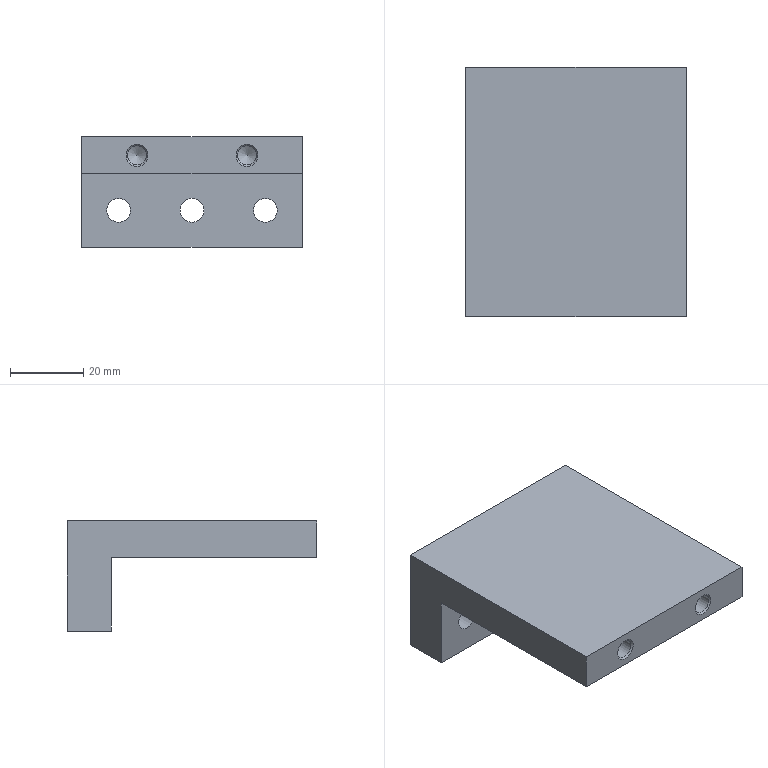Part | NX | features SIMPLE HOLE 5, DATUM_CSYS 4, SKETCH 3, HOLE PACKAGE 2, SYMBOLIC_THREAD 2, EXTRUDE 1 | 1 solid | 17 faces | box 60 x 68 x 30 mm | volume 53216 mm3 | plane 8 | cylinder 5 | cone 4 | commonest cylinder face diameters 6.5 x3 5.2 x2
STEP:
#1=CARTESIAN_POINT('',(15.,-68.,28.));
#2=VERTEX_POINT('',#1);
#3=CARTESIAN_POINT('',(15.,-68.,25.));
#4=DIRECTION('',(0.,1.,0.));
#5=DIRECTION('',(0.,0.,1.));
#6=AXIS2_PLACEMENT_3D('',#3,#4,#5);
#7=CIRCLE('',#6,3.);
#8=EDGE_CURVE('',#2,#2,#7,.T.);
#9=ORIENTED_EDGE('',*,*,#8,.T.);
#10=EDGE_LOOP('',(#9));
#11=FACE_BOUND('',#10,.T.);
#12=CARTESIAN_POINT('',(-15.,-68.,28.));
#13=VERTEX_POINT('',#12);
#14=CARTESIAN_POINT('',(-15.,-68.,25.));
#15=DIRECTION('',(0.,1.,0.));
#16=DIRECTION('',(0.,0.,1.));
#17=AXIS2_PLACEMENT_3D('',#14,#15,#16);
#18=CIRCLE('',#17,3.);
#19=EDGE_CURVE('',#13,#13,#18,.T.);
#20=ORIENTED_EDGE('',*,*,#19,.T.);
#21=EDGE_LOOP('',(#20));
#22=FACE_BOUND('',#21,.T.);
#23=CARTESIAN_POINT('',(-30.,-68.,30.));
#24=VERTEX_POINT('',#23);
#25=CARTESIAN_POINT('',(-30.,-68.,20.));
#26=VERTEX_POINT('',#25);
#27=CARTESIAN_POINT('',(-30.,-68.,30.));
#28=DIRECTION('',(0.,0.,-1.));
#29=VECTOR('',#28,1000.);
#30=LINE('',#27,#29);
#31=EDGE_CURVE('',#24,#26,#30,.T.);
#32=ORIENTED_EDGE('',*,*,#31,.T.);
#33=CARTESIAN_POINT('',(30.,-68.,20.));
#34=VERTEX_POINT('',#33);
#35=CARTESIAN_POINT('',(30.,-68.,20.));
#36=DIRECTION('',(-1.,0.,0.));
#37=VECTOR('',#36,1000.);
#38=LINE('',#35,#37);
#39=EDGE_CURVE('',#34,#26,#38,.T.);
#40=ORIENTED_EDGE('',*,*,#39,.F.);
#41=CARTESIAN_POINT('',(30.,-68.,30.));
#42=VERTEX_POINT('',#41);
#43=CARTESIAN_POINT('',(30.,-68.,30.));
#44=DIRECTION('',(0.,0.,-1.));
#45=VECTOR('',#44,1000.);
#46=LINE('',#43,#45);
#47=EDGE_CURVE('',#42,#34,#46,.T.);
#48=ORIENTED_EDGE('',*,*,#47,.F.);
#49=CARTESIAN_POINT('',(30.,-68.,30.));
#50=DIRECTION('',(-1.,0.,0.));
#51=VECTOR('',#50,1000.);
#52=LINE('',#49,#51);
#53=EDGE_CURVE('',#42,#24,#52,.T.);
#54=ORIENTED_EDGE('',*,*,#53,.T.);
#55=EDGE_LOOP('',(#32,#40,#48,#54));
#56=FACE_BOUND('',#55,.T.);
#57=CARTESIAN_POINT('',(30.,-68.,30.));
#58=DIRECTION('',(0.,1.,0.));
#59=DIRECTION('',(0.,0.,1.));
#60=AXIS2_PLACEMENT_3D('',#57,#58,#59);
#61=PLANE('',#60);
#62=ADVANCED_FACE('',(#11,#22,#56),#61,.F.);
#63=CARTESIAN_POINT('',(-30.,-12.,20.));
#64=VERTEX_POINT('',#63);
#65=CARTESIAN_POINT('',(-30.,-68.,20.));
#66=DIRECTION('',(0.,1.,0.));
#67=VECTOR('',#66,1000.);
#68=LINE('',#65,#67);
#69=EDGE_CURVE('',#26,#64,#68,.T.);
#70=ORIENTED_EDGE('',*,*,#69,.T.);
#71=CARTESIAN_POINT('',(30.,-12.,20.));
#72=VERTEX_POINT('',#71);
#73=CARTESIAN_POINT('',(30.,-12.,20.));
#74=DIRECTION('',(-1.,0.,0.));
#75=VECTOR('',#74,1000.);
#76=LINE('',#73,#75);
#77=EDGE_CURVE('',#72,#64,#76,.T.);
#78=ORIENTED_EDGE('',*,*,#77,.F.);
#79=CARTESIAN_POINT('',(30.,-68.,20.));
#80=DIRECTION('',(0.,1.,0.));
#81=VECTOR('',#80,1000.);
#82=LINE('',#79,#81);
#83=EDGE_CURVE('',#34,#72,#82,.T.);
#84=ORIENTED_EDGE('',*,*,#83,.F.);
#85=ORIENTED_EDGE('',*,*,#39,.T.);
#86=EDGE_LOOP('',(#70,#78,#84,#85));
#87=FACE_BOUND('',#86,.T.);
#88=CARTESIAN_POINT('',(30.,-68.,20.));
#89=DIRECTION('',(0.,0.,1.));
#90=DIRECTION('',(1.,0.,0.));
#91=AXIS2_PLACEMENT_3D('',#88,#89,#90);
#92=PLANE('',#91);
#93=ADVANCED_FACE('',(#87),#92,.F.);
#94=CARTESIAN_POINT('',(-20.,-12.,13.25));
#95=VERTEX_POINT('',#94);
#96=CARTESIAN_POINT('',(-20.,-12.,10.));
#97=DIRECTION('',(0.,1.,0.));
#98=DIRECTION('',(0.,0.,1.));
#99=AXIS2_PLACEMENT_3D('',#96,#97,#98);
#100=CIRCLE('',#99,3.25);
#101=EDGE_CURVE('',#95,#95,#100,.T.);
#102=ORIENTED_EDGE('',*,*,#101,.T.);
#103=EDGE_LOOP('',(#102));
#104=FACE_BOUND('',#103,.T.);
#105=CARTESIAN_POINT('',(0.,-12.,13.25));
#106=VERTEX_POINT('',#105);
#107=CARTESIAN_POINT('',(0.,-12.,10.));
#108=DIRECTION('',(0.,1.,0.));
#109=DIRECTION('',(0.,0.,1.));
#110=AXIS2_PLACEMENT_3D('',#107,#108,#109);
#111=CIRCLE('',#110,3.25);
#112=EDGE_CURVE('',#106,#106,#111,.T.);
#113=ORIENTED_EDGE('',*,*,#112,.T.);
#114=EDGE_LOOP('',(#113));
#115=FACE_BOUND('',#114,.T.);
#116=CARTESIAN_POINT('',(20.,-12.,13.25));
#117=VERTEX_POINT('',#116);
#118=CARTESIAN_POINT('',(20.,-12.,10.));
#119=DIRECTION('',(0.,1.,0.));
#120=DIRECTION('',(0.,0.,1.));
#121=AXIS2_PLACEMENT_3D('',#118,#119,#120);
#122=CIRCLE('',#121,3.25);
#123=EDGE_CURVE('',#117,#117,#122,.T.);
#124=ORIENTED_EDGE('',*,*,#123,.T.);
#125=EDGE_LOOP('',(#124));
#126=FACE_BOUND('',#125,.T.);
#127=CARTESIAN_POINT('',(-30.,-12.,0.));
#128=VERTEX_POINT('',#127);
#129=CARTESIAN_POINT('',(-30.,-12.,20.));
#130=DIRECTION('',(0.,0.,-1.));
#131=VECTOR('',#130,1000.);
#132=LINE('',#129,#131);
#133=EDGE_CURVE('',#64,#128,#132,.T.);
#134=ORIENTED_EDGE('',*,*,#133,.T.);
#135=CARTESIAN_POINT('',(30.,-12.,0.));
#136=VERTEX_POINT('',#135);
#137=CARTESIAN_POINT('',(30.,-12.,0.));
#138=DIRECTION('',(-1.,0.,0.));
#139=VECTOR('',#138,1000.);
#140=LINE('',#137,#139);
#141=EDGE_CURVE('',#136,#128,#140,.T.);
#142=ORIENTED_EDGE('',*,*,#141,.F.);
#143=CARTESIAN_POINT('',(30.,-12.,20.));
#144=DIRECTION('',(0.,0.,-1.));
#145=VECTOR('',#144,1000.);
#146=LINE('',#143,#145);
#147=EDGE_CURVE('',#72,#136,#146,.T.);
#148=ORIENTED_EDGE('',*,*,#147,.F.);
#149=ORIENTED_EDGE('',*,*,#77,.T.);
#150=EDGE_LOOP('',(#134,#142,#148,#149));
#151=FACE_BOUND('',#150,.T.);
#152=CARTESIAN_POINT('',(30.,-12.,20.));
#153=DIRECTION('',(0.,1.,0.));
#154=DIRECTION('',(0.,0.,1.));
#155=AXIS2_PLACEMENT_3D('',#152,#153,#154);
#156=PLANE('',#155);
#157=ADVANCED_FACE('',(#104,#115,#126,#151),#156,.F.);
#158=CARTESIAN_POINT('',(-30.,0.,0.));
#159=VERTEX_POINT('',#158);
#160=CARTESIAN_POINT('',(-30.,-12.,0.));
#161=DIRECTION('',(0.,1.,0.));
#162=VECTOR('',#161,1000.);
#163=LINE('',#160,#162);
#164=EDGE_CURVE('',#128,#159,#163,.T.);
#165=ORIENTED_EDGE('',*,*,#164,.T.);
#166=CARTESIAN_POINT('',(30.,0.,0.));
#167=VERTEX_POINT('',#166);
#168=CARTESIAN_POINT('',(30.,0.,0.));
#169=DIRECTION('',(-1.,0.,0.));
#170=VECTOR('',#169,1000.);
#171=LINE('',#168,#170);
#172=EDGE_CURVE('',#167,#159,#171,.T.);
#173=ORIENTED_EDGE('',*,*,#172,.F.);
#174=CARTESIAN_POINT('',(30.,-12.,0.));
#175=DIRECTION('',(0.,1.,0.));
#176=VECTOR('',#175,1000.);
#177=LINE('',#174,#176);
#178=EDGE_CURVE('',#136,#167,#177,.T.);
#179=ORIENTED_EDGE('',*,*,#178,.F.);
#180=ORIENTED_EDGE('',*,*,#141,.T.);
#181=EDGE_LOOP('',(#165,#173,#179,#180));
#182=FACE_BOUND('',#181,.T.);
#183=CARTESIAN_POINT('',(30.,-12.,0.));
#184=DIRECTION('',(0.,0.,1.));
#185=DIRECTION('',(1.,0.,0.));
#186=AXIS2_PLACEMENT_3D('',#183,#184,#185);
#187=PLANE('',#186);
#188=ADVANCED_FACE('',(#182),#187,.F.);
#189=CARTESIAN_POINT('',(-20.,0.,6.75));
#190=VERTEX_POINT('',#189);
#191=CARTESIAN_POINT('',(-20.,0.,10.));
#192=DIRECTION('',(0.,-1.,0.));
#193=DIRECTION('',(0.,0.,-1.));
#194=AXIS2_PLACEMENT_3D('',#191,#192,#193);
#195=CIRCLE('',#194,3.25);
#196=EDGE_CURVE('',#190,#190,#195,.T.);
#197=ORIENTED_EDGE('',*,*,#196,.T.);
#198=EDGE_LOOP('',(#197));
#199=FACE_BOUND('',#198,.T.);
#200=CARTESIAN_POINT('',(0.,0.,6.75));
#201=VERTEX_POINT('',#200);
#202=CARTESIAN_POINT('',(0.,0.,10.));
#203=DIRECTION('',(0.,-1.,0.));
#204=DIRECTION('',(0.,0.,-1.));
#205=AXIS2_PLACEMENT_3D('',#202,#203,#204);
#206=CIRCLE('',#205,3.25);
#207=EDGE_CURVE('',#201,#201,#206,.T.);
#208=ORIENTED_EDGE('',*,*,#207,.T.);
#209=EDGE_LOOP('',(#208));
#210=FACE_BOUND('',#209,.T.);
#211=CARTESIAN_POINT('',(20.,0.,6.75));
#212=VERTEX_POINT('',#211);
#213=CARTESIAN_POINT('',(20.,0.,10.));
#214=DIRECTION('',(0.,-1.,0.));
#215=DIRECTION('',(0.,0.,-1.));
#216=AXIS2_PLACEMENT_3D('',#213,#214,#215);
#217=CIRCLE('',#216,3.25);
#218=EDGE_CURVE('',#212,#212,#217,.T.);
#219=ORIENTED_EDGE('',*,*,#218,.T.);
#220=EDGE_LOOP('',(#219));
#221=FACE_BOUND('',#220,.T.);
#222=CARTESIAN_POINT('',(-30.,0.,30.));
#223=VERTEX_POINT('',#222);
#224=CARTESIAN_POINT('',(-30.,0.,0.));
#225=DIRECTION('',(0.,0.,1.));
#226=VECTOR('',#225,1000.);
#227=LINE('',#224,#226);
#228=EDGE_CURVE('',#159,#223,#227,.T.);
#229=ORIENTED_EDGE('',*,*,#228,.T.);
#230=CARTESIAN_POINT('',(30.,0.,30.));
#231=VERTEX_POINT('',#230);
#232=CARTESIAN_POINT('',(30.,0.,30.));
#233=DIRECTION('',(-1.,0.,0.));
#234=VECTOR('',#233,1000.);
#235=LINE('',#232,#234);
#236=EDGE_CURVE('',#231,#223,#235,.T.);
#237=ORIENTED_EDGE('',*,*,#236,.F.);
#238=CARTESIAN_POINT('',(30.,0.,0.));
#239=DIRECTION('',(0.,0.,1.));
#240=VECTOR('',#239,1000.);
#241=LINE('',#238,#240);
#242=EDGE_CURVE('',#167,#231,#241,.T.);
#243=ORIENTED_EDGE('',*,*,#242,.F.);
#244=ORIENTED_EDGE('',*,*,#172,.T.);
#245=EDGE_LOOP('',(#229,#237,#243,#244));
#246=FACE_BOUND('',#245,.T.);
#247=CARTESIAN_POINT('',(30.,0.,0.));
#248=DIRECTION('',(0.,-1.,0.));
#249=DIRECTION('',(0.,0.,-1.));
#250=AXIS2_PLACEMENT_3D('',#247,#248,#249);
#251=PLANE('',#250);
#252=ADVANCED_FACE('',(#199,#210,#221,#246),#251,.F.);
#253=CARTESIAN_POINT('',(-30.,0.,30.));
#254=DIRECTION('',(0.,-1.,0.));
#255=VECTOR('',#254,1000.);
#256=LINE('',#253,#255);
#257=EDGE_CURVE('',#223,#24,#256,.T.);
#258=ORIENTED_EDGE('',*,*,#257,.T.);
#259=ORIENTED_EDGE('',*,*,#53,.F.);
#260=CARTESIAN_POINT('',(30.,0.,30.));
#261=DIRECTION('',(0.,-1.,0.));
#262=VECTOR('',#261,1000.);
#263=LINE('',#260,#262);
#264=EDGE_CURVE('',#231,#42,#263,.T.);
#265=ORIENTED_EDGE('',*,*,#264,.F.);
#266=ORIENTED_EDGE('',*,*,#236,.T.);
#267=EDGE_LOOP('',(#258,#259,#265,#266));
#268=FACE_BOUND('',#267,.T.);
#269=CARTESIAN_POINT('',(30.,0.,30.));
#270=DIRECTION('',(0.,0.,-1.));
#271=DIRECTION('',(0.,1.,0.));
#272=AXIS2_PLACEMENT_3D('',#269,#270,#271);
#273=PLANE('',#272);
#274=ADVANCED_FACE('',(#268),#273,.F.);
#275=ORIENTED_EDGE('',*,*,#47,.T.);
#276=ORIENTED_EDGE('',*,*,#83,.T.);
#277=ORIENTED_EDGE('',*,*,#147,.T.);
#278=ORIENTED_EDGE('',*,*,#178,.T.);
#279=ORIENTED_EDGE('',*,*,#242,.T.);
#280=ORIENTED_EDGE('',*,*,#264,.T.);
#281=EDGE_LOOP('',(#275,#276,#277,#278,#279,#280));
#282=FACE_BOUND('',#281,.T.);
#283=CARTESIAN_POINT('',(30.,0.,0.));
#284=DIRECTION('',(1.,0.,0.));
#285=DIRECTION('',(0.,0.,-1.));
#286=AXIS2_PLACEMENT_3D('',#283,#284,#285);
#287=PLANE('',#286);
#288=ADVANCED_FACE('',(#282),#287,.T.);
#289=ORIENTED_EDGE('',*,*,#31,.F.);
#290=ORIENTED_EDGE('',*,*,#257,.F.);
#291=ORIENTED_EDGE('',*,*,#228,.F.);
#292=ORIENTED_EDGE('',*,*,#164,.F.);
#293=ORIENTED_EDGE('',*,*,#133,.F.);
#294=ORIENTED_EDGE('',*,*,#69,.F.);
#295=EDGE_LOOP('',(#289,#290,#291,#292,#293,#294));
#296=FACE_BOUND('',#295,.T.);
#297=CARTESIAN_POINT('',(-30.,0.,0.));
#298=DIRECTION('',(1.,0.,0.));
#299=DIRECTION('',(0.,0.,-1.));
#300=AXIS2_PLACEMENT_3D('',#297,#298,#299);
#301=PLANE('',#300);
#302=ADVANCED_FACE('',(#296),#301,.F.);
#303=CARTESIAN_POINT('',(-15.,-50.,27.6));
#304=VERTEX_POINT('',#303);
#305=CARTESIAN_POINT('',(-15.,-50.,25.));
#306=DIRECTION('',(0.,1.,0.));
#307=DIRECTION('',(0.,0.,1.));
#308=AXIS2_PLACEMENT_3D('',#305,#306,#307);
#309=CIRCLE('',#308,2.6);
#310=EDGE_CURVE('',#304,#304,#309,.F.);
#311=ORIENTED_EDGE('',*,*,#310,.T.);
#312=EDGE_LOOP('',(#311));
#313=FACE_BOUND('',#312,.T.);
#314=CARTESIAN_POINT('',(-15.,-48.438,25.));
#315=VERTEX_POINT('',#314);
#316=VERTEX_LOOP('',#315);
#317=FACE_BOUND('',#316,.T.);
#318=CARTESIAN_POINT('',(-15.,-50.,25.));
#319=DIRECTION('',(0.,-1.,0.));
#320=DIRECTION('',(0.,0.,-1.));
#321=AXIS2_PLACEMENT_3D('',#318,#319,#320);
#322=CONICAL_SURFACE('',#321,2.6,1.03);
#323=ADVANCED_FACE('',(#313,#317),#322,.F.);
#324=CARTESIAN_POINT('',(-15.,-67.6,27.6));
#325=VERTEX_POINT('',#324);
#326=CARTESIAN_POINT('',(-15.,-67.6,25.));
#327=DIRECTION('',(0.,1.,0.));
#328=DIRECTION('',(0.,0.,1.));
#329=AXIS2_PLACEMENT_3D('',#326,#327,#328);
#330=CIRCLE('',#329,2.6);
#331=EDGE_CURVE('',#325,#325,#330,.F.);
#332=ORIENTED_EDGE('',*,*,#331,.T.);
#333=EDGE_LOOP('',(#332));
#334=FACE_BOUND('',#333,.T.);
#335=ORIENTED_EDGE('',*,*,#310,.F.);
#336=EDGE_LOOP('',(#335));
#337=FACE_BOUND('',#336,.T.);
#338=CARTESIAN_POINT('',(-15.,-68.,25.));
#339=DIRECTION('',(0.,1.,0.));
#340=DIRECTION('',(0.,0.,1.));
#341=AXIS2_PLACEMENT_3D('',#338,#339,#340);
#342=CYLINDRICAL_SURFACE('',#341,2.6);
#343=ADVANCED_FACE('',(#334,#337),#342,.F.);
#344=ORIENTED_EDGE('',*,*,#331,.F.);
#345=EDGE_LOOP('',(#344));
#346=FACE_BOUND('',#345,.T.);
#347=ORIENTED_EDGE('',*,*,#19,.F.);
#348=EDGE_LOOP('',(#347));
#349=FACE_BOUND('',#348,.T.);
#350=CARTESIAN_POINT('',(-15.,-68.,25.));
#351=DIRECTION('',(0.,-1.,0.));
#352=DIRECTION('',(0.,0.,-1.));
#353=AXIS2_PLACEMENT_3D('',#350,#351,#352);
#354=CONICAL_SURFACE('',#353,3.,0.7854);
#355=ADVANCED_FACE('',(#346,#349),#354,.F.);
#356=CARTESIAN_POINT('',(15.,-50.,27.6));
#357=VERTEX_POINT('',#356);
#358=CARTESIAN_POINT('',(15.,-50.,25.));
#359=DIRECTION('',(0.,1.,0.));
#360=DIRECTION('',(0.,0.,1.));
#361=AXIS2_PLACEMENT_3D('',#358,#359,#360);
#362=CIRCLE('',#361,2.6);
#363=EDGE_CURVE('',#357,#357,#362,.F.);
#364=ORIENTED_EDGE('',*,*,#363,.T.);
#365=EDGE_LOOP('',(#364));
#366=FACE_BOUND('',#365,.T.);
#367=CARTESIAN_POINT('',(15.,-48.438,25.));
#368=VERTEX_POINT('',#367);
#369=VERTEX_LOOP('',#368);
#370=FACE_BOUND('',#369,.T.);
#371=CARTESIAN_POINT('',(15.,-50.,25.));
#372=DIRECTION('',(0.,-1.,0.));
#373=DIRECTION('',(0.,0.,-1.));
#374=AXIS2_PLACEMENT_3D('',#371,#372,#373);
#375=CONICAL_SURFACE('',#374,2.6,1.03);
#376=ADVANCED_FACE('',(#366,#370),#375,.F.);
#377=CARTESIAN_POINT('',(15.,-67.6,27.6));
#378=VERTEX_POINT('',#377);
#379=CARTESIAN_POINT('',(15.,-67.6,25.));
#380=DIRECTION('',(0.,1.,0.));
#381=DIRECTION('',(0.,0.,1.));
#382=AXIS2_PLACEMENT_3D('',#379,#380,#381);
#383=CIRCLE('',#382,2.6);
#384=EDGE_CURVE('',#378,#378,#383,.F.);
#385=ORIENTED_EDGE('',*,*,#384,.T.);
#386=EDGE_LOOP('',(#385));
#387=FACE_BOUND('',#386,.T.);
#388=ORIENTED_EDGE('',*,*,#363,.F.);
#389=EDGE_LOOP('',(#388));
#390=FACE_BOUND('',#389,.T.);
#391=CARTESIAN_POINT('',(15.,-68.,25.));
#392=DIRECTION('',(0.,1.,0.));
#393=DIRECTION('',(0.,0.,1.));
#394=AXIS2_PLACEMENT_3D('',#391,#392,#393);
#395=CYLINDRICAL_SURFACE('',#394,2.6);
#396=ADVANCED_FACE('',(#387,#390),#395,.F.);
#397=ORIENTED_EDGE('',*,*,#384,.F.);
#398=EDGE_LOOP('',(#397));
#399=FACE_BOUND('',#398,.T.);
#400=ORIENTED_EDGE('',*,*,#8,.F.);
#401=EDGE_LOOP('',(#400));
#402=FACE_BOUND('',#401,.T.);
#403=CARTESIAN_POINT('',(15.,-68.,25.));
#404=DIRECTION('',(0.,-1.,0.));
#405=DIRECTION('',(0.,0.,-1.));
#406=AXIS2_PLACEMENT_3D('',#403,#404,#405);
#407=CONICAL_SURFACE('',#406,3.,0.7854);
#408=ADVANCED_FACE('',(#399,#402),#407,.F.);
#409=ORIENTED_EDGE('',*,*,#123,.F.);
#410=EDGE_LOOP('',(#409));
#411=FACE_BOUND('',#410,.T.);
#412=ORIENTED_EDGE('',*,*,#218,.F.);
#413=EDGE_LOOP('',(#412));
#414=FACE_BOUND('',#413,.T.);
#415=CARTESIAN_POINT('',(20.,-12.,10.));
#416=DIRECTION('',(0.,1.,0.));
#417=DIRECTION('',(0.,0.,1.));
#418=AXIS2_PLACEMENT_3D('',#415,#416,#417);
#419=CYLINDRICAL_SURFACE('',#418,3.25);
#420=ADVANCED_FACE('',(#411,#414),#419,.F.);
#421=ORIENTED_EDGE('',*,*,#112,.F.);
#422=EDGE_LOOP('',(#421));
#423=FACE_BOUND('',#422,.T.);
#424=ORIENTED_EDGE('',*,*,#207,.F.);
#425=EDGE_LOOP('',(#424));
#426=FACE_BOUND('',#425,.T.);
#427=CARTESIAN_POINT('',(0.,-12.,10.));
#428=DIRECTION('',(0.,1.,0.));
#429=DIRECTION('',(0.,0.,1.));
#430=AXIS2_PLACEMENT_3D('',#427,#428,#429);
#431=CYLINDRICAL_SURFACE('',#430,3.25);
#432=ADVANCED_FACE('',(#423,#426),#431,.F.);
#433=ORIENTED_EDGE('',*,*,#101,.F.);
#434=EDGE_LOOP('',(#433));
#435=FACE_BOUND('',#434,.T.);
#436=ORIENTED_EDGE('',*,*,#196,.F.);
#437=EDGE_LOOP('',(#436));
#438=FACE_BOUND('',#437,.T.);
#439=CARTESIAN_POINT('',(-20.,-12.,10.));
#440=DIRECTION('',(0.,1.,0.));
#441=DIRECTION('',(0.,0.,1.));
#442=AXIS2_PLACEMENT_3D('',#439,#440,#441);
#443=CYLINDRICAL_SURFACE('',#442,3.25);
#444=ADVANCED_FACE('',(#435,#438),#443,.F.);
#445=CLOSED_SHELL('',(#62,#93,#157,#188,#252,#274,#288,#302,#323,#343,#355,#376,#396,#408,#420,#432,#444));
#446=MANIFOLD_SOLID_BREP('',#445);
#447=(LENGTH_UNIT()NAMED_UNIT(*)SI_UNIT(.MILLI.,.METRE.));
#448=UNCERTAINTY_MEASURE_WITH_UNIT(LENGTH_MEASURE(0.00001),#447,'','');
#449=(NAMED_UNIT(*)PLANE_ANGLE_UNIT()SI_UNIT($,.RADIAN.));
#450=(NAMED_UNIT(*)SI_UNIT($,.STERADIAN.)SOLID_ANGLE_UNIT());
#451=(GEOMETRIC_REPRESENTATION_CONTEXT(3)GLOBAL_UNCERTAINTY_ASSIGNED_CONTEXT((#448))GLOBAL_UNIT_ASSIGNED_CONTEXT((#447,#449,#450))REPRESENTATION_CONTEXT('',''));
#452=ADVANCED_BREP_SHAPE_REPRESENTATION('',(#446),#451);